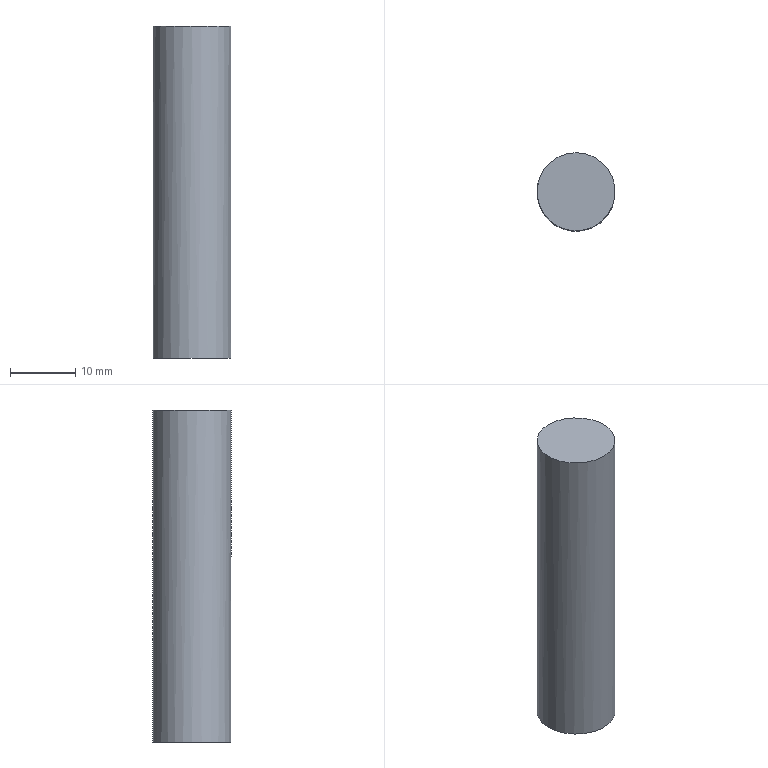Part | STEP file | solid 82 | 1 solid | 3 faces | box 12 x 12 x 51 mm | volume 5768 mm3 | plane 2 | cylinder 1 | commonest cylinder face diameters 12 x1